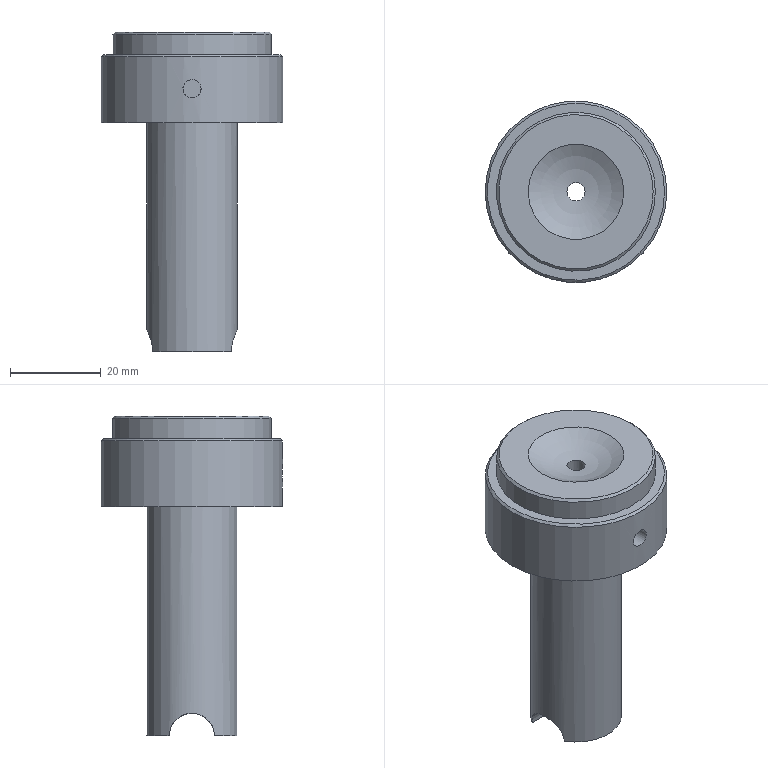Part | NX | features 模具.stp<1>[83] 2 | 1 solid | 15 faces | box 40 x 40 x 70.5 mm | volume 35720 mm3 | plane 6 | cylinder 5 | cone 3 | sphere 1 | commonest cylinder face diameters 4 x1 10 x1 20 x1 35 x1 40 x1
STEP:
#1=CARTESIAN_POINT('',(-1.745,-4.536,42.103));
#2=VERTEX_POINT('',#1);
#3=CARTESIAN_POINT('',(-3.187,-3.694,43.473));
#4=CARTESIAN_POINT('',(-2.258,-4.347,42.569));
#5=CARTESIAN_POINT('',(-1.409,-4.668,41.797));
#6=CARTESIAN_POINT('',(-1.188,-4.739,41.601));
#7=CARTESIAN_POINT('',(-0.8276,-4.827,41.31));
#8=CARTESIAN_POINT('',(-0.6361,-4.864,41.164));
#9=CARTESIAN_POINT('',(-0.2986,-4.905,40.975));
#10=CARTESIAN_POINT('',(-0.01143,-4.913,40.925));
#11=CARTESIAN_POINT('',(0.258,-4.907,40.963));
#12=CARTESIAN_POINT('',(0.5956,-4.87,41.135));
#13=CARTESIAN_POINT('',(0.7649,-4.84,41.262));
#14=CARTESIAN_POINT('',(1.134,-4.755,41.555));
#15=CARTESIAN_POINT('',(1.374,-4.68,41.766));
#16=CARTESIAN_POINT('',(1.893,-4.488,42.236));
#17=CARTESIAN_POINT('',(2.578,-4.116,42.885));
#18=CARTESIAN_POINT('',(3.254,-3.566,43.541));
#19=CARTESIAN_POINT('',(3.818,-2.902,44.097));
#20=CARTESIAN_POINT('',(4.231,-2.233,44.504));
#21=CARTESIAN_POINT('',(4.615,-1.247,44.884));
#22=CARTESIAN_POINT('',(4.759,-0.1821,45.033));
#23=CARTESIAN_POINT('',(4.694,0.8772,44.965));
#24=CARTESIAN_POINT('',(4.26,2.303,44.53));
#25=CARTESIAN_POINT('',(3.481,3.419,43.763));
#26=CARTESIAN_POINT('',(2.365,4.297,42.67));
#27=CARTESIAN_POINT('',(1.366,4.687,41.757));
#28=CARTESIAN_POINT('',(1.076,4.772,41.503));
#29=CARTESIAN_POINT('',(0.6822,4.854,41.204));
#30=CARTESIAN_POINT('',(0.4856,4.884,41.074));
#31=CARTESIAN_POINT('',(0.259,4.904,40.974));
#32=CARTESIAN_POINT('',(0.0798,4.911,40.939));
#33=CARTESIAN_POINT('',(-0.12,4.911,40.94));
#34=CARTESIAN_POINT('',(-0.3127,4.903,40.986));
#35=CARTESIAN_POINT('',(-0.6395,4.864,41.162));
#36=CARTESIAN_POINT('',(-0.7973,4.833,41.286));
#37=CARTESIAN_POINT('',(-1.164,4.747,41.581));
#38=CARTESIAN_POINT('',(-1.403,4.671,41.791));
#39=CARTESIAN_POINT('',(-1.912,4.479,42.254));
#40=CARTESIAN_POINT('',(-2.595,4.105,42.901));
#41=CARTESIAN_POINT('',(-3.264,3.555,43.551));
#42=CARTESIAN_POINT('',(-3.824,2.893,44.103));
#43=CARTESIAN_POINT('',(-4.234,2.227,44.507));
#44=CARTESIAN_POINT('',(-4.614,1.246,44.884));
#45=CARTESIAN_POINT('',(-4.758,0.1868,45.032));
#46=CARTESIAN_POINT('',(-4.695,-0.8629,44.967));
#47=CARTESIAN_POINT('',(-4.368,-1.958,44.639));
#48=CARTESIAN_POINT('',(-3.942,-2.727,44.219));
#49=CARTESIAN_POINT('',(-3.187,-3.694,43.473));
#50=CARTESIAN_POINT('',(-2.258,-4.347,42.569));
#51=CARTESIAN_POINT('',(-1.409,-4.668,41.797));
#52=B_SPLINE_CURVE_WITH_KNOTS('',3,(#3,#4,#5,#6,#7,#8,#9,#10,#11,#12,#13,#14,#15,#16,#17,#18,#19,#20,#21,#22,#23,#24,#25,#26,#27,#28,#29,#30,#31,#32,#33,#34,#35,#36,#37,#38,#39,#40,#41,#42,#43,#44,#45,#46,#47,#48,#49,#50,#51),.UNSPECIFIED.,.T.,.F.,(1,1,1,1,1,1,1,1,1,1,1,1,1,1,1,1,1,1,1,1,1,1,1,1,1,1,1,1,1,1,1,1,1,1,1,1,1,1,1,1,1,1,1,1,1,1,1,1,1,1,1,1,1),(-0.1316,-0.09867,-0.06578,0.,0.01188,0.02375,0.03325,0.04275,0.05213,0.06151,0.07046,0.07941,0.08834,0.09727,0.1104,0.1236,0.1536,0.1836,0.2137,0.2437,0.2749,0.3061,0.3372,0.3684,0.4309,0.4934,0.5114,0.5294,0.5377,0.546,0.5543,0.5584,0.5623,0.5709,0.5795,0.5884,0.5973,0.6104,0.6236,0.6536,0.6836,0.7137,0.7437,0.7749,0.8061,0.8372,0.8684,0.9013,0.9342,1.,1.012,1.024,1.033),.UNSPECIFIED.);
#53=EDGE_CURVE('',#2,#2,#52,.T.);
#54=ORIENTED_EDGE('',*,*,#53,.T.);
#55=EDGE_LOOP('',(#54));
#56=FACE_BOUND('',#55,.T.);
#57=CARTESIAN_POINT('',(8.66,5.,40.));
#58=VERTEX_POINT('',#57);
#59=CARTESIAN_POINT('',(-8.66,5.,40.));
#60=VERTEX_POINT('',#59);
#61=CARTESIAN_POINT('',(87.,5.,40.));
#62=DIRECTION('',(-1.,0.,0.));
#63=VECTOR('',#62,1000.);
#64=LINE('',#61,#63);
#65=EDGE_CURVE('',#58,#60,#64,.T.);
#66=ORIENTED_EDGE('',*,*,#65,.F.);
#67=CARTESIAN_POINT('',(8.66,-5.,40.));
#68=VERTEX_POINT('',#67);
#69=CARTESIAN_POINT('',(8.66,5.,40.));
#70=CARTESIAN_POINT('',(8.66,5.,40.298));
#71=CARTESIAN_POINT('',(8.69,4.956,40.778));
#72=CARTESIAN_POINT('',(8.775,4.808,41.415));
#73=CARTESIAN_POINT('',(8.887,4.596,41.987));
#74=CARTESIAN_POINT('',(8.948,4.477,42.234));
#75=CARTESIAN_POINT('',(9.058,4.252,42.647));
#76=CARTESIAN_POINT('',(9.187,3.963,43.068));
#77=CARTESIAN_POINT('',(9.416,3.391,43.715));
#78=CARTESIAN_POINT('',(9.588,2.853,44.129));
#79=CARTESIAN_POINT('',(9.729,2.295,44.448));
#80=CARTESIAN_POINT('',(9.802,1.961,44.608));
#81=CARTESIAN_POINT('',(9.897,1.419,44.805));
#82=CARTESIAN_POINT('',(9.975,0.7732,44.957));
#83=CARTESIAN_POINT('',(10.017,-0.008245,45.029));
#84=CARTESIAN_POINT('',(9.974,-0.7869,44.955));
#85=CARTESIAN_POINT('',(9.896,-1.43,44.802));
#86=CARTESIAN_POINT('',(9.801,-1.97,44.604));
#87=CARTESIAN_POINT('',(9.728,-2.3,44.446));
#88=CARTESIAN_POINT('',(9.587,-2.855,44.127));
#89=CARTESIAN_POINT('',(9.415,-3.393,43.713));
#90=CARTESIAN_POINT('',(9.186,-3.963,43.068));
#91=CARTESIAN_POINT('',(9.058,-4.252,42.646));
#92=CARTESIAN_POINT('',(8.948,-4.477,42.234));
#93=CARTESIAN_POINT('',(8.887,-4.596,41.986));
#94=CARTESIAN_POINT('',(8.775,-4.808,41.415));
#95=CARTESIAN_POINT('',(8.69,-4.956,40.778));
#96=CARTESIAN_POINT('',(8.66,-5.,40.298));
#97=CARTESIAN_POINT('',(8.66,-5.,40.));
#98=B_SPLINE_CURVE_WITH_KNOTS('',3,(#69,#70,#71,#72,#73,#74,#75,#76,#77,#78,#79,#80,#81,#82,#83,#84,#85,#86,#87,#88,#89,#90,#91,#92,#93,#94,#95,#96,#97),.UNSPECIFIED.,.F.,.F.,(4,1,1,1,1,1,1,1,1,1,1,1,1,1,1,1,1,1,1,1,1,1,1,1,1,1,4),(0.,0.0625,0.09375,0.125,0.1562,0.1875,0.2188,0.25,0.3125,0.3438,0.375,0.4062,0.4375,0.5,0.5625,0.5938,0.625,0.6562,0.6875,0.75,0.7812,0.8125,0.8438,0.875,0.9062,0.9375,1.),.UNSPECIFIED.);
#99=EDGE_CURVE('',#68,#58,#98,.F.);
#100=ORIENTED_EDGE('',*,*,#99,.F.);
#101=CARTESIAN_POINT('',(-8.66,-5.,40.));
#102=VERTEX_POINT('',#101);
#103=CARTESIAN_POINT('',(87.,-5.,40.));
#104=DIRECTION('',(1.,0.,0.));
#105=VECTOR('',#104,1000.);
#106=LINE('',#103,#105);
#107=EDGE_CURVE('',#102,#68,#106,.T.);
#108=ORIENTED_EDGE('',*,*,#107,.F.);
#109=CARTESIAN_POINT('',(-8.66,-5.,40.));
#110=CARTESIAN_POINT('',(-8.66,-5.,40.298));
#111=CARTESIAN_POINT('',(-8.69,-4.956,40.778));
#112=CARTESIAN_POINT('',(-8.775,-4.808,41.415));
#113=CARTESIAN_POINT('',(-8.887,-4.596,41.987));
#114=CARTESIAN_POINT('',(-8.948,-4.477,42.234));
#115=CARTESIAN_POINT('',(-9.058,-4.252,42.647));
#116=CARTESIAN_POINT('',(-9.187,-3.963,43.068));
#117=CARTESIAN_POINT('',(-9.416,-3.391,43.715));
#118=CARTESIAN_POINT('',(-9.588,-2.853,44.129));
#119=CARTESIAN_POINT('',(-9.729,-2.295,44.448));
#120=CARTESIAN_POINT('',(-9.802,-1.961,44.608));
#121=CARTESIAN_POINT('',(-9.897,-1.419,44.805));
#122=CARTESIAN_POINT('',(-9.975,-0.7732,44.957));
#123=CARTESIAN_POINT('',(-10.017,0.008245,45.029));
#124=CARTESIAN_POINT('',(-9.974,0.7869,44.955));
#125=CARTESIAN_POINT('',(-9.896,1.43,44.802));
#126=CARTESIAN_POINT('',(-9.801,1.97,44.604));
#127=CARTESIAN_POINT('',(-9.728,2.3,44.446));
#128=CARTESIAN_POINT('',(-9.587,2.855,44.127));
#129=CARTESIAN_POINT('',(-9.415,3.393,43.713));
#130=CARTESIAN_POINT('',(-9.186,3.963,43.068));
#131=CARTESIAN_POINT('',(-9.058,4.252,42.646));
#132=CARTESIAN_POINT('',(-8.948,4.477,42.234));
#133=CARTESIAN_POINT('',(-8.887,4.596,41.986));
#134=CARTESIAN_POINT('',(-8.775,4.808,41.415));
#135=CARTESIAN_POINT('',(-8.69,4.956,40.778));
#136=CARTESIAN_POINT('',(-8.66,5.,40.298));
#137=CARTESIAN_POINT('',(-8.66,5.,40.));
#138=B_SPLINE_CURVE_WITH_KNOTS('',3,(#109,#110,#111,#112,#113,#114,#115,#116,#117,#118,#119,#120,#121,#122,#123,#124,#125,#126,#127,#128,#129,#130,#131,#132,#133,#134,#135,#136,#137),.UNSPECIFIED.,.F.,.F.,(4,1,1,1,1,1,1,1,1,1,1,1,1,1,1,1,1,1,1,1,1,1,1,1,1,1,4),(0.,0.0625,0.09375,0.125,0.1562,0.1875,0.2188,0.25,0.3125,0.3438,0.375,0.4062,0.4375,0.5,0.5625,0.5938,0.625,0.6562,0.6875,0.75,0.7812,0.8125,0.8438,0.875,0.9062,0.9375,1.),.UNSPECIFIED.);
#139=EDGE_CURVE('',#60,#102,#138,.F.);
#140=ORIENTED_EDGE('',*,*,#139,.F.);
#141=EDGE_LOOP('',(#66,#100,#108,#140));
#142=FACE_BOUND('',#141,.T.);
#143=CARTESIAN_POINT('',(87.,0.,40.));
#144=DIRECTION('',(1.,0.,0.));
#145=DIRECTION('',(0.,1.,0.));
#146=AXIS2_PLACEMENT_3D('',#143,#144,#145);
#147=CYLINDRICAL_SURFACE('',#146,5.);
#148=ADVANCED_FACE('',(#56,#142),#147,.F.);
#149=CARTESIAN_POINT('',(2.,0.,107.6));
#150=VERTEX_POINT('',#149);
#151=CARTESIAN_POINT('',(0.,0.,107.6));
#152=DIRECTION('',(0.,0.,1.));
#153=DIRECTION('',(1.,0.,0.));
#154=AXIS2_PLACEMENT_3D('',#151,#152,#153);
#155=CIRCLE('',#154,2.);
#156=EDGE_CURVE('',#150,#150,#155,.T.);
#157=ORIENTED_EDGE('',*,*,#156,.F.);
#158=EDGE_LOOP('',(#157));
#159=FACE_BOUND('',#158,.T.);
#160=CARTESIAN_POINT('',(10.536,0.,110.5));
#161=VERTEX_POINT('',#160);
#162=CARTESIAN_POINT('',(0.,0.,110.5));
#163=DIRECTION('',(0.,0.,1.));
#164=DIRECTION('',(1.,0.,0.));
#165=AXIS2_PLACEMENT_3D('',#162,#163,#164);
#166=CIRCLE('',#165,10.536);
#167=EDGE_CURVE('',#161,#161,#166,.T.);
#168=ORIENTED_EDGE('',*,*,#167,.T.);
#169=EDGE_LOOP('',(#168));
#170=FACE_BOUND('',#169,.T.);
#171=CARTESIAN_POINT('',(0.,0.,127.5));
#172=DIRECTION('',(0.,0.,1.));
#173=DIRECTION('',(1.,0.,0.));
#174=AXIS2_PLACEMENT_3D('',#171,#172,#173);
#175=SPHERICAL_SURFACE('',#174,20.);
#176=ADVANCED_FACE('',(#159,#170),#175,.F.);
#177=CARTESIAN_POINT('',(2.,-14.,98.));
#178=VERTEX_POINT('',#177);
#179=CARTESIAN_POINT('',(0.,-14.,98.));
#180=DIRECTION('',(0.,1.,0.));
#181=DIRECTION('',(1.,0.,0.));
#182=AXIS2_PLACEMENT_3D('',#179,#180,#181);
#183=CIRCLE('',#182,2.);
#184=EDGE_CURVE('',#178,#178,#183,.T.);
#185=ORIENTED_EDGE('',*,*,#184,.T.);
#186=EDGE_LOOP('',(#185));
#187=FACE_BOUND('',#186,.T.);
#188=CARTESIAN_POINT('',(-1.988,-19.901,98.22));
#189=VERTEX_POINT('',#188);
#190=CARTESIAN_POINT('',(-1.93,-19.907,98.584));
#191=CARTESIAN_POINT('',(-2.021,-19.897,98.128));
#192=CARTESIAN_POINT('',(-1.974,-19.902,97.558));
#193=CARTESIAN_POINT('',(-1.829,-19.917,97.161));
#194=CARTESIAN_POINT('',(-1.593,-19.937,96.763));
#195=CARTESIAN_POINT('',(-1.317,-19.957,96.478));
#196=CARTESIAN_POINT('',(-0.8872,-19.982,96.175));
#197=CARTESIAN_POINT('',(-0.2641,-20.004,95.96));
#198=CARTESIAN_POINT('',(0.4266,-19.998,96.023));
#199=CARTESIAN_POINT('',(0.837,-19.983,96.17));
#200=CARTESIAN_POINT('',(1.236,-19.963,96.406));
#201=CARTESIAN_POINT('',(1.521,-19.943,96.683));
#202=CARTESIAN_POINT('',(1.825,-19.917,97.11));
#203=CARTESIAN_POINT('',(1.976,-19.902,97.575));
#204=CARTESIAN_POINT('',(2.018,-19.898,98.141));
#205=CARTESIAN_POINT('',(1.916,-19.908,98.638));
#206=CARTESIAN_POINT('',(1.752,-19.923,98.981));
#207=CARTESIAN_POINT('',(1.514,-19.944,99.342));
#208=CARTESIAN_POINT('',(1.112,-19.97,99.677));
#209=CARTESIAN_POINT('',(0.8939,-19.981,99.798));
#210=CARTESIAN_POINT('',(0.5041,-19.995,99.949));
#211=CARTESIAN_POINT('',(0.03978,-20.003,100.025));
#212=CARTESIAN_POINT('',(-0.5101,-19.996,99.961));
#213=CARTESIAN_POINT('',(-0.9056,-19.98,99.79));
#214=CARTESIAN_POINT('',(-1.242,-19.963,99.601));
#215=CARTESIAN_POINT('',(-1.653,-19.933,99.152));
#216=CARTESIAN_POINT('',(-1.743,-19.924,98.993));
#217=CARTESIAN_POINT('',(-1.93,-19.907,98.584));
#218=CARTESIAN_POINT('',(-2.021,-19.897,98.128));
#219=CARTESIAN_POINT('',(-1.974,-19.902,97.558));
#220=B_SPLINE_CURVE_WITH_KNOTS('',3,(#190,#191,#192,#193,#194,#195,#196,#197,#198,#199,#200,#201,#202,#203,#204,#205,#206,#207,#208,#209,#210,#211,#212,#213,#214,#215,#216,#217,#218,#219),.UNSPECIFIED.,.T.,.F.,(1,1,1,1,1,1,1,1,1,1,1,1,1,1,1,1,1,1,1,1,1,1,1,1,1,1,1,1,1,1,1,1,1,1),(-0.09362,-0.06347,-0.03174,0.,0.05937,0.09055,0.1217,0.1545,0.1859,0.2468,0.3092,0.3405,0.3717,0.4045,0.4359,0.4968,0.5166,0.5748,0.6049,0.635,0.6652,0.6953,0.7255,0.7556,0.8159,0.8461,0.8762,0.9064,0.9365,0.9683,1.,1.059,1.091,1.122),.UNSPECIFIED.);
#221=EDGE_CURVE('',#189,#189,#220,.T.);
#222=ORIENTED_EDGE('',*,*,#221,.T.);
#223=EDGE_LOOP('',(#222));
#224=FACE_BOUND('',#223,.T.);
#225=CARTESIAN_POINT('',(0.,-14.,98.));
#226=DIRECTION('',(0.,-1.,0.));
#227=DIRECTION('',(1.,0.,0.));
#228=AXIS2_PLACEMENT_3D('',#225,#226,#227);
#229=CYLINDRICAL_SURFACE('',#228,2.);
#230=ADVANCED_FACE('',(#187,#224),#229,.F.);
#231=ORIENTED_EDGE('',*,*,#184,.F.);
#232=EDGE_LOOP('',(#231));
#233=FACE_BOUND('',#232,.T.);
#234=CARTESIAN_POINT('',(0.,-14.,98.));
#235=DIRECTION('',(0.,1.,0.));
#236=DIRECTION('',(1.,0.,0.));
#237=AXIS2_PLACEMENT_3D('',#234,#235,#236);
#238=PLANE('',#237);
#239=ADVANCED_FACE('',(#233),#238,.F.);
#240=CARTESIAN_POINT('',(20.,0.,105.));
#241=VERTEX_POINT('',#240);
#242=CARTESIAN_POINT('',(0.,0.,105.));
#243=DIRECTION('',(0.,0.,-1.));
#244=DIRECTION('',(1.,0.,0.));
#245=AXIS2_PLACEMENT_3D('',#242,#243,#244);
#246=CIRCLE('',#245,20.);
#247=EDGE_CURVE('',#241,#241,#246,.T.);
#248=ORIENTED_EDGE('',*,*,#247,.F.);
#249=EDGE_LOOP('',(#248));
#250=FACE_BOUND('',#249,.T.);
#251=CARTESIAN_POINT('',(19.5,0.,105.5));
#252=VERTEX_POINT('',#251);
#253=CARTESIAN_POINT('',(0.,0.,105.5));
#254=DIRECTION('',(0.,0.,1.));
#255=DIRECTION('',(1.,0.,0.));
#256=AXIS2_PLACEMENT_3D('',#253,#254,#255);
#257=CIRCLE('',#256,19.5);
#258=EDGE_CURVE('',#252,#252,#257,.T.);
#259=ORIENTED_EDGE('',*,*,#258,.F.);
#260=EDGE_LOOP('',(#259));
#261=FACE_BOUND('',#260,.T.);
#262=CARTESIAN_POINT('',(0.,0.,105.));
#263=DIRECTION('',(0.,0.,-1.));
#264=DIRECTION('',(-1.,0.,0.));
#265=AXIS2_PLACEMENT_3D('',#262,#263,#264);
#266=CONICAL_SURFACE('',#265,20.,0.7854);
#267=ADVANCED_FACE('',(#250,#261),#266,.T.);
#268=ORIENTED_EDGE('',*,*,#247,.T.);
#269=EDGE_LOOP('',(#268));
#270=FACE_BOUND('',#269,.T.);
#271=ORIENTED_EDGE('',*,*,#221,.F.);
#272=EDGE_LOOP('',(#271));
#273=FACE_BOUND('',#272,.T.);
#274=CARTESIAN_POINT('',(-20.,0.,90.5));
#275=VERTEX_POINT('',#274);
#276=CARTESIAN_POINT('',(0.,0.,90.5));
#277=DIRECTION('',(0.,0.,-1.));
#278=DIRECTION('',(-1.,0.,0.));
#279=AXIS2_PLACEMENT_3D('',#276,#277,#278);
#280=CIRCLE('',#279,20.);
#281=EDGE_CURVE('',#275,#275,#280,.T.);
#282=ORIENTED_EDGE('',*,*,#281,.F.);
#283=EDGE_LOOP('',(#282));
#284=FACE_BOUND('',#283,.T.);
#285=CARTESIAN_POINT('',(0.,0.,80.5));
#286=DIRECTION('',(0.,0.,1.));
#287=DIRECTION('',(1.,0.,0.));
#288=AXIS2_PLACEMENT_3D('',#285,#286,#287);
#289=CYLINDRICAL_SURFACE('',#288,20.);
#290=ADVANCED_FACE('',(#270,#273,#284),#289,.T.);
#291=ORIENTED_EDGE('',*,*,#258,.T.);
#292=EDGE_LOOP('',(#291));
#293=FACE_BOUND('',#292,.T.);
#294=CARTESIAN_POINT('',(17.5,0.,105.5));
#295=VERTEX_POINT('',#294);
#296=CARTESIAN_POINT('',(0.,0.,105.5));
#297=DIRECTION('',(0.,0.,-1.));
#298=DIRECTION('',(1.,0.,0.));
#299=AXIS2_PLACEMENT_3D('',#296,#297,#298);
#300=CIRCLE('',#299,17.5);
#301=EDGE_CURVE('',#295,#295,#300,.T.);
#302=ORIENTED_EDGE('',*,*,#301,.T.);
#303=EDGE_LOOP('',(#302));
#304=FACE_BOUND('',#303,.T.);
#305=CARTESIAN_POINT('',(0.,0.,105.5));
#306=DIRECTION('',(0.,0.,1.));
#307=DIRECTION('',(1.,0.,0.));
#308=AXIS2_PLACEMENT_3D('',#305,#306,#307);
#309=PLANE('',#308);
#310=ADVANCED_FACE('',(#293,#304),#309,.T.);
#311=CARTESIAN_POINT('',(17.5,0.,110.));
#312=VERTEX_POINT('',#311);
#313=CARTESIAN_POINT('',(0.,0.,110.));
#314=DIRECTION('',(0.,0.,-1.));
#315=DIRECTION('',(1.,0.,0.));
#316=AXIS2_PLACEMENT_3D('',#313,#314,#315);
#317=CIRCLE('',#316,17.5);
#318=EDGE_CURVE('',#312,#312,#317,.T.);
#319=ORIENTED_EDGE('',*,*,#318,.F.);
#320=EDGE_LOOP('',(#319));
#321=FACE_BOUND('',#320,.T.);
#322=CARTESIAN_POINT('',(17.,0.,110.5));
#323=VERTEX_POINT('',#322);
#324=CARTESIAN_POINT('',(0.,0.,110.5));
#325=DIRECTION('',(0.,0.,1.));
#326=DIRECTION('',(1.,0.,0.));
#327=AXIS2_PLACEMENT_3D('',#324,#325,#326);
#328=CIRCLE('',#327,17.);
#329=EDGE_CURVE('',#323,#323,#328,.T.);
#330=ORIENTED_EDGE('',*,*,#329,.F.);
#331=EDGE_LOOP('',(#330));
#332=FACE_BOUND('',#331,.T.);
#333=CARTESIAN_POINT('',(0.,0.,110.));
#334=DIRECTION('',(0.,0.,-1.));
#335=DIRECTION('',(-1.,0.,0.));
#336=AXIS2_PLACEMENT_3D('',#333,#334,#335);
#337=CONICAL_SURFACE('',#336,17.5,0.7854);
#338=ADVANCED_FACE('',(#321,#332),#337,.T.);
#339=ORIENTED_EDGE('',*,*,#301,.F.);
#340=EDGE_LOOP('',(#339));
#341=FACE_BOUND('',#340,.T.);
#342=ORIENTED_EDGE('',*,*,#318,.T.);
#343=EDGE_LOOP('',(#342));
#344=FACE_BOUND('',#343,.T.);
#345=CARTESIAN_POINT('',(0.,0.,105.));
#346=DIRECTION('',(0.,0.,1.));
#347=DIRECTION('',(1.,0.,0.));
#348=AXIS2_PLACEMENT_3D('',#345,#346,#347);
#349=CYLINDRICAL_SURFACE('',#348,17.5);
#350=ADVANCED_FACE('',(#341,#344),#349,.T.);
#351=ORIENTED_EDGE('',*,*,#329,.T.);
#352=EDGE_LOOP('',(#351));
#353=FACE_BOUND('',#352,.T.);
#354=ORIENTED_EDGE('',*,*,#167,.F.);
#355=EDGE_LOOP('',(#354));
#356=FACE_BOUND('',#355,.T.);
#357=CARTESIAN_POINT('',(0.,0.,110.5));
#358=DIRECTION('',(0.,0.,1.));
#359=DIRECTION('',(1.,0.,0.));
#360=AXIS2_PLACEMENT_3D('',#357,#358,#359);
#361=PLANE('',#360);
#362=ADVANCED_FACE('',(#353,#356),#361,.T.);
#363=ORIENTED_EDGE('',*,*,#281,.T.);
#364=EDGE_LOOP('',(#363));
#365=FACE_BOUND('',#364,.T.);
#366=CARTESIAN_POINT('',(-10.,0.,90.5));
#367=VERTEX_POINT('',#366);
#368=CARTESIAN_POINT('',(0.,0.,90.5));
#369=DIRECTION('',(0.,0.,-1.));
#370=DIRECTION('',(-1.,0.,0.));
#371=AXIS2_PLACEMENT_3D('',#368,#369,#370);
#372=CIRCLE('',#371,10.);
#373=EDGE_CURVE('',#367,#367,#372,.T.);
#374=ORIENTED_EDGE('',*,*,#373,.F.);
#375=EDGE_LOOP('',(#374));
#376=FACE_BOUND('',#375,.T.);
#377=CARTESIAN_POINT('',(0.,0.,90.5));
#378=DIRECTION('',(0.,0.,-1.));
#379=DIRECTION('',(0.,-1.,0.));
#380=AXIS2_PLACEMENT_3D('',#377,#378,#379);
#381=PLANE('',#380);
#382=ADVANCED_FACE('',(#365,#376),#381,.T.);
#383=CARTESIAN_POINT('',(0.,0.,40.));
#384=DIRECTION('',(0.,0.,1.));
#385=DIRECTION('',(-1.,0.,0.));
#386=AXIS2_PLACEMENT_3D('',#383,#384,#385);
#387=CIRCLE('',#386,10.);
#388=EDGE_CURVE('',#102,#68,#387,.T.);
#389=ORIENTED_EDGE('',*,*,#388,.F.);
#390=ORIENTED_EDGE('',*,*,#107,.T.);
#391=EDGE_LOOP('',(#389,#390));
#392=FACE_BOUND('',#391,.T.);
#393=CARTESIAN_POINT('',(9.88,-84.073,40.));
#394=DIRECTION('',(0.,0.,-1.));
#395=DIRECTION('',(0.,-1.,0.));
#396=AXIS2_PLACEMENT_3D('',#393,#394,#395);
#397=PLANE('',#396);
#398=ADVANCED_FACE('',(#392),#397,.T.);
#399=CARTESIAN_POINT('',(0.,0.,40.));
#400=DIRECTION('',(0.,0.,1.));
#401=DIRECTION('',(-1.,0.,0.));
#402=AXIS2_PLACEMENT_3D('',#399,#400,#401);
#403=CIRCLE('',#402,10.);
#404=EDGE_CURVE('',#58,#60,#403,.T.);
#405=ORIENTED_EDGE('',*,*,#404,.F.);
#406=ORIENTED_EDGE('',*,*,#65,.T.);
#407=EDGE_LOOP('',(#405,#406));
#408=FACE_BOUND('',#407,.T.);
#409=CARTESIAN_POINT('',(9.88,-84.073,40.));
#410=DIRECTION('',(0.,0.,-1.));
#411=DIRECTION('',(0.,-1.,0.));
#412=AXIS2_PLACEMENT_3D('',#409,#410,#411);
#413=PLANE('',#412);
#414=ADVANCED_FACE('',(#408),#413,.T.);
#415=ORIENTED_EDGE('',*,*,#53,.F.);
#416=EDGE_LOOP('',(#415));
#417=FACE_BOUND('',#416,.T.);
#418=ORIENTED_EDGE('',*,*,#156,.T.);
#419=EDGE_LOOP('',(#418));
#420=FACE_BOUND('',#419,.T.);
#421=CARTESIAN_POINT('',(0.,0.,107.6));
#422=DIRECTION('',(0.,0.,-1.));
#423=DIRECTION('',(1.,0.,0.));
#424=AXIS2_PLACEMENT_3D('',#421,#422,#423);
#425=CONICAL_SURFACE('',#424,2.,0.04363);
#426=ADVANCED_FACE('',(#417,#420),#425,.F.);
#427=ORIENTED_EDGE('',*,*,#388,.T.);
#428=ORIENTED_EDGE('',*,*,#99,.T.);
#429=ORIENTED_EDGE('',*,*,#404,.T.);
#430=ORIENTED_EDGE('',*,*,#139,.T.);
#431=EDGE_LOOP('',(#427,#428,#429,#430));
#432=FACE_BOUND('',#431,.T.);
#433=ORIENTED_EDGE('',*,*,#373,.T.);
#434=EDGE_LOOP('',(#433));
#435=FACE_BOUND('',#434,.T.);
#436=CARTESIAN_POINT('',(0.,0.,80.5));
#437=DIRECTION('',(0.,0.,-1.));
#438=DIRECTION('',(1.,0.,0.));
#439=AXIS2_PLACEMENT_3D('',#436,#437,#438);
#440=CYLINDRICAL_SURFACE('',#439,10.);
#441=ADVANCED_FACE('',(#432,#435),#440,.T.);
#442=CLOSED_SHELL('',(#148,#176,#230,#239,#267,#290,#310,#338,#350,#362,#382,#398,#414,#426,#441));
#443=MANIFOLD_SOLID_BREP('',#442);
#444=(LENGTH_UNIT()NAMED_UNIT(*)SI_UNIT(.MILLI.,.METRE.));
#445=UNCERTAINTY_MEASURE_WITH_UNIT(LENGTH_MEASURE(0.0508),#444,'','');
#446=(NAMED_UNIT(*)PLANE_ANGLE_UNIT()SI_UNIT($,.RADIAN.));
#447=(NAMED_UNIT(*)SI_UNIT($,.STERADIAN.)SOLID_ANGLE_UNIT());
#448=(GEOMETRIC_REPRESENTATION_CONTEXT(3)GLOBAL_UNCERTAINTY_ASSIGNED_CONTEXT((#445))GLOBAL_UNIT_ASSIGNED_CONTEXT((#444,#446,#447))REPRESENTATION_CONTEXT('',''));
#449=ADVANCED_BREP_SHAPE_REPRESENTATION('',(#443),#448);